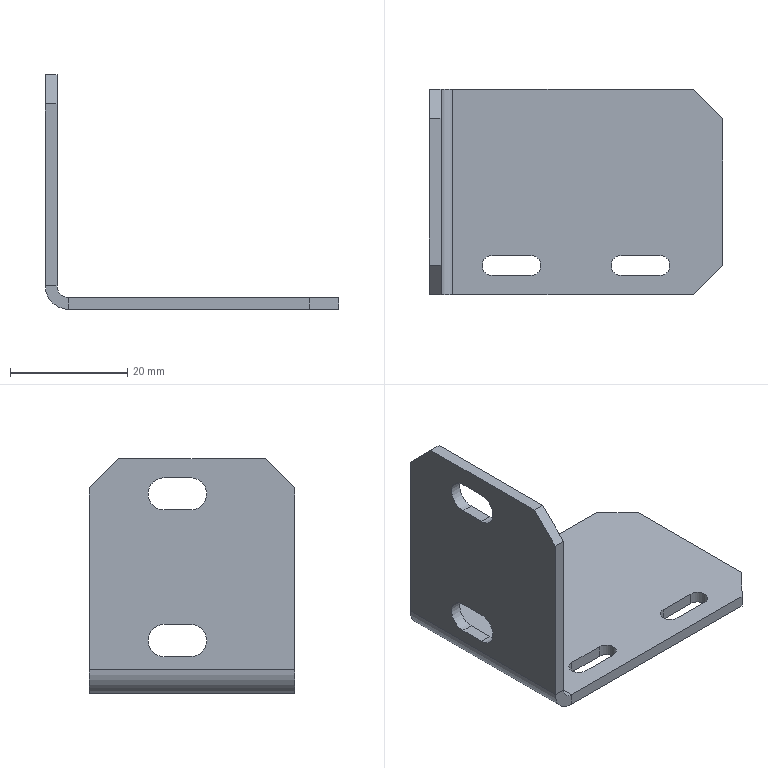Part | SolidWorks | features HoleWzd 2, Chamfer 1, EdgeFlange 1, FlatPattern 1, SMBaseFlange 1, SheetMetal 1 | 1 solid | 34 faces | box 50 x 35 x 40 mm | volume 5650 mm3 | plane 24 | cylinder 10 | commonest cylinder face diameters 3.4 x4 5.5 x4 4 x1 8 x1
STEP:
#1=CARTESIAN_POINT('',(48.,12.5,-20.));
#2=VERTEX_POINT('',#1);
#3=CARTESIAN_POINT('',(48.,-12.5,-20.));
#4=VERTEX_POINT('',#3);
#5=CARTESIAN_POINT('',(48.,0.,-20.));
#6=DIRECTION('',(0.,-1.,0.));
#7=VECTOR('',#6,1000.);
#8=LINE('',#5,#7);
#9=EDGE_CURVE('',#2,#4,#8,.T.);
#10=ORIENTED_EDGE('',*,*,#9,.T.);
#11=CARTESIAN_POINT('',(43.,-17.5,-20.));
#12=VERTEX_POINT('',#11);
#13=CARTESIAN_POINT('',(43.,-17.5,-20.));
#14=DIRECTION('',(-0.7071,-0.7071,0.));
#15=VECTOR('',#14,1000.);
#16=LINE('',#13,#15);
#17=EDGE_CURVE('',#4,#12,#16,.T.);
#18=ORIENTED_EDGE('',*,*,#17,.T.);
#19=CARTESIAN_POINT('',(2.,-17.5,-20.));
#20=VERTEX_POINT('',#19);
#21=CARTESIAN_POINT('',(0.,-17.5,-20.));
#22=DIRECTION('',(-1.,0.,0.));
#23=VECTOR('',#22,1000.);
#24=LINE('',#21,#23);
#25=EDGE_CURVE('',#12,#20,#24,.T.);
#26=ORIENTED_EDGE('',*,*,#25,.T.);
#27=CARTESIAN_POINT('',(2.,17.5,-20.));
#28=VERTEX_POINT('',#27);
#29=CARTESIAN_POINT('',(2.,-17.5,-20.));
#30=DIRECTION('',(0.,-1.,0.));
#31=VECTOR('',#30,1000.);
#32=LINE('',#29,#31);
#33=EDGE_CURVE('',#28,#20,#32,.T.);
#34=ORIENTED_EDGE('',*,*,#33,.F.);
#35=CARTESIAN_POINT('',(43.,17.5,-20.));
#36=VERTEX_POINT('',#35);
#37=CARTESIAN_POINT('',(0.,17.5,-20.));
#38=DIRECTION('',(1.,0.,0.));
#39=VECTOR('',#38,1000.);
#40=LINE('',#37,#39);
#41=EDGE_CURVE('',#28,#36,#40,.T.);
#42=ORIENTED_EDGE('',*,*,#41,.T.);
#43=CARTESIAN_POINT('',(48.,12.5,-20.));
#44=DIRECTION('',(0.7071,-0.7071,0.));
#45=VECTOR('',#44,1000.);
#46=LINE('',#43,#45);
#47=EDGE_CURVE('',#36,#2,#46,.T.);
#48=ORIENTED_EDGE('',*,*,#47,.T.);
#49=EDGE_LOOP('',(#10,#18,#26,#34,#42,#48));
#50=FACE_OUTER_BOUND('',#49,.T.);
#51=CARTESIAN_POINT('',(15.3,-10.8,-20.));
#52=VERTEX_POINT('',#51);
#53=CARTESIAN_POINT('',(8.7,-10.8,-20.));
#54=VERTEX_POINT('',#53);
#55=CARTESIAN_POINT('',(15.3,-10.8,-20.));
#56=DIRECTION('',(-1.,0.,0.));
#57=VECTOR('',#56,1000.);
#58=LINE('',#55,#57);
#59=EDGE_CURVE('',#52,#54,#58,.T.);
#60=ORIENTED_EDGE('',*,*,#59,.T.);
#61=CARTESIAN_POINT('',(8.7,-14.2,-20.));
#62=VERTEX_POINT('',#61);
#63=CARTESIAN_POINT('',(8.7,-12.5,-20.));
#64=DIRECTION('',(0.,0.,-1.));
#65=DIRECTION('',(0.,1.,0.));
#66=AXIS2_PLACEMENT_3D('',#63,#64,#65);
#67=CIRCLE('',#66,1.7);
#68=EDGE_CURVE('',#62,#54,#67,.T.);
#69=ORIENTED_EDGE('',*,*,#68,.F.);
#70=CARTESIAN_POINT('',(15.3,-14.2,-20.));
#71=VERTEX_POINT('',#70);
#72=CARTESIAN_POINT('',(15.3,-14.2,-20.));
#73=DIRECTION('',(-1.,0.,0.));
#74=VECTOR('',#73,1000.);
#75=LINE('',#72,#74);
#76=EDGE_CURVE('',#71,#62,#75,.T.);
#77=ORIENTED_EDGE('',*,*,#76,.F.);
#78=CARTESIAN_POINT('',(15.3,-12.5,-20.));
#79=DIRECTION('',(0.,0.,-1.));
#80=DIRECTION('',(0.,1.,0.));
#81=AXIS2_PLACEMENT_3D('',#78,#79,#80);
#82=CIRCLE('',#81,1.7);
#83=EDGE_CURVE('',#52,#71,#82,.T.);
#84=ORIENTED_EDGE('',*,*,#83,.F.);
#85=EDGE_LOOP('',(#60,#69,#77,#84));
#86=FACE_BOUND('',#85,.T.);
#87=CARTESIAN_POINT('',(37.3,-10.8,-20.));
#88=VERTEX_POINT('',#87);
#89=CARTESIAN_POINT('',(37.3,-14.2,-20.));
#90=VERTEX_POINT('',#89);
#91=CARTESIAN_POINT('',(37.3,-12.5,-20.));
#92=DIRECTION('',(0.,0.,-1.));
#93=DIRECTION('',(0.,1.,0.));
#94=AXIS2_PLACEMENT_3D('',#91,#92,#93);
#95=CIRCLE('',#94,1.7);
#96=EDGE_CURVE('',#88,#90,#95,.T.);
#97=ORIENTED_EDGE('',*,*,#96,.F.);
#98=CARTESIAN_POINT('',(30.7,-10.8,-20.));
#99=VERTEX_POINT('',#98);
#100=CARTESIAN_POINT('',(37.3,-10.8,-20.));
#101=DIRECTION('',(-1.,0.,0.));
#102=VECTOR('',#101,1000.);
#103=LINE('',#100,#102);
#104=EDGE_CURVE('',#88,#99,#103,.T.);
#105=ORIENTED_EDGE('',*,*,#104,.T.);
#106=CARTESIAN_POINT('',(30.7,-14.2,-20.));
#107=VERTEX_POINT('',#106);
#108=CARTESIAN_POINT('',(30.7,-12.5,-20.));
#109=DIRECTION('',(0.,0.,-1.));
#110=DIRECTION('',(0.,1.,0.));
#111=AXIS2_PLACEMENT_3D('',#108,#109,#110);
#112=CIRCLE('',#111,1.7);
#113=EDGE_CURVE('',#107,#99,#112,.T.);
#114=ORIENTED_EDGE('',*,*,#113,.F.);
#115=CARTESIAN_POINT('',(37.3,-14.2,-20.));
#116=DIRECTION('',(-1.,0.,0.));
#117=VECTOR('',#116,1000.);
#118=LINE('',#115,#117);
#119=EDGE_CURVE('',#90,#107,#118,.T.);
#120=ORIENTED_EDGE('',*,*,#119,.F.);
#121=EDGE_LOOP('',(#97,#105,#114,#120));
#122=FACE_BOUND('',#121,.T.);
#123=CARTESIAN_POINT('',(0.,0.,-20.));
#124=DIRECTION('',(0.,0.,1.));
#125=DIRECTION('',(1.,0.,0.));
#126=AXIS2_PLACEMENT_3D('',#123,#124,#125);
#127=PLANE('',#126);
#128=ADVANCED_FACE('',(#50,#86,#122),#127,.F.);
#129=CARTESIAN_POINT('',(-2.,17.5,-16.));
#130=VERTEX_POINT('',#129);
#131=CARTESIAN_POINT('',(-2.,17.5,15.));
#132=VERTEX_POINT('',#131);
#133=CARTESIAN_POINT('',(-2.,17.5,20.));
#134=DIRECTION('',(0.,0.,1.));
#135=VECTOR('',#134,1000.);
#136=LINE('',#133,#135);
#137=EDGE_CURVE('',#130,#132,#136,.T.);
#138=ORIENTED_EDGE('',*,*,#137,.T.);
#139=CARTESIAN_POINT('',(0.,17.5,15.));
#140=VERTEX_POINT('',#139);
#141=CARTESIAN_POINT('',(-2.,17.5,15.));
#142=DIRECTION('',(1.,0.,0.));
#143=VECTOR('',#142,1000.);
#144=LINE('',#141,#143);
#145=EDGE_CURVE('',#132,#140,#144,.T.);
#146=ORIENTED_EDGE('',*,*,#145,.T.);
#147=CARTESIAN_POINT('',(0.,17.5,-16.));
#148=VERTEX_POINT('',#147);
#149=CARTESIAN_POINT('',(0.,17.5,20.));
#150=DIRECTION('',(0.,0.,1.));
#151=VECTOR('',#150,1000.);
#152=LINE('',#149,#151);
#153=EDGE_CURVE('',#148,#140,#152,.T.);
#154=ORIENTED_EDGE('',*,*,#153,.F.);
#155=CARTESIAN_POINT('',(0.,17.5,-16.));
#156=DIRECTION('',(-1.,0.,0.));
#157=VECTOR('',#156,1000.);
#158=LINE('',#155,#157);
#159=EDGE_CURVE('',#148,#130,#158,.T.);
#160=ORIENTED_EDGE('',*,*,#159,.T.);
#161=EDGE_LOOP('',(#138,#146,#154,#160));
#162=FACE_OUTER_BOUND('',#161,.T.);
#163=CARTESIAN_POINT('',(-2.,17.5,20.));
#164=DIRECTION('',(0.,1.,0.));
#165=DIRECTION('',(0.,0.,1.));
#166=AXIS2_PLACEMENT_3D('',#163,#164,#165);
#167=PLANE('',#166);
#168=ADVANCED_FACE('',(#162),#167,.T.);
#169=CARTESIAN_POINT('',(-2.,4.75,16.75));
#170=VERTEX_POINT('',#169);
#171=CARTESIAN_POINT('',(-2.,0.25,16.75));
#172=VERTEX_POINT('',#171);
#173=CARTESIAN_POINT('',(-2.,4.75,16.75));
#174=DIRECTION('',(0.,-1.,0.));
#175=VECTOR('',#174,1000.);
#176=LINE('',#173,#175);
#177=EDGE_CURVE('',#170,#172,#176,.T.);
#178=ORIENTED_EDGE('',*,*,#177,.T.);
#179=CARTESIAN_POINT('',(-2.,0.25,11.25));
#180=VERTEX_POINT('',#179);
#181=CARTESIAN_POINT('',(-2.,0.25,14.));
#182=DIRECTION('',(1.,0.,0.));
#183=DIRECTION('',(0.,0.,-1.));
#184=AXIS2_PLACEMENT_3D('',#181,#182,#183);
#185=CIRCLE('',#184,2.75);
#186=EDGE_CURVE('',#172,#180,#185,.T.);
#187=ORIENTED_EDGE('',*,*,#186,.T.);
#188=CARTESIAN_POINT('',(-2.,4.75,11.25));
#189=VERTEX_POINT('',#188);
#190=CARTESIAN_POINT('',(-2.,4.75,11.25));
#191=DIRECTION('',(0.,-1.,0.));
#192=VECTOR('',#191,1000.);
#193=LINE('',#190,#192);
#194=EDGE_CURVE('',#189,#180,#193,.T.);
#195=ORIENTED_EDGE('',*,*,#194,.F.);
#196=CARTESIAN_POINT('',(-2.,4.75,14.));
#197=DIRECTION('',(1.,0.,0.));
#198=DIRECTION('',(0.,0.,-1.));
#199=AXIS2_PLACEMENT_3D('',#196,#197,#198);
#200=CIRCLE('',#199,2.75);
#201=EDGE_CURVE('',#189,#170,#200,.T.);
#202=ORIENTED_EDGE('',*,*,#201,.T.);
#203=EDGE_LOOP('',(#178,#187,#195,#202));
#204=FACE_BOUND('',#203,.T.);
#205=CARTESIAN_POINT('',(-2.,4.75,-8.25));
#206=VERTEX_POINT('',#205);
#207=CARTESIAN_POINT('',(-2.,0.25,-8.25));
#208=VERTEX_POINT('',#207);
#209=CARTESIAN_POINT('',(-2.,4.75,-8.25));
#210=DIRECTION('',(0.,-1.,0.));
#211=VECTOR('',#210,1000.);
#212=LINE('',#209,#211);
#213=EDGE_CURVE('',#206,#208,#212,.T.);
#214=ORIENTED_EDGE('',*,*,#213,.T.);
#215=CARTESIAN_POINT('',(-2.,0.25,-13.75));
#216=VERTEX_POINT('',#215);
#217=CARTESIAN_POINT('',(-2.,0.25,-11.));
#218=DIRECTION('',(1.,0.,0.));
#219=DIRECTION('',(0.,0.,-1.));
#220=AXIS2_PLACEMENT_3D('',#217,#218,#219);
#221=CIRCLE('',#220,2.75);
#222=EDGE_CURVE('',#208,#216,#221,.T.);
#223=ORIENTED_EDGE('',*,*,#222,.T.);
#224=CARTESIAN_POINT('',(-2.,4.75,-13.75));
#225=VERTEX_POINT('',#224);
#226=CARTESIAN_POINT('',(-2.,4.75,-13.75));
#227=DIRECTION('',(0.,-1.,0.));
#228=VECTOR('',#227,1000.);
#229=LINE('',#226,#228);
#230=EDGE_CURVE('',#225,#216,#229,.T.);
#231=ORIENTED_EDGE('',*,*,#230,.F.);
#232=CARTESIAN_POINT('',(-2.,4.75,-11.));
#233=DIRECTION('',(1.,0.,0.));
#234=DIRECTION('',(0.,0.,-1.));
#235=AXIS2_PLACEMENT_3D('',#232,#233,#234);
#236=CIRCLE('',#235,2.75);
#237=EDGE_CURVE('',#225,#206,#236,.T.);
#238=ORIENTED_EDGE('',*,*,#237,.T.);
#239=EDGE_LOOP('',(#214,#223,#231,#238));
#240=FACE_BOUND('',#239,.T.);
#241=CARTESIAN_POINT('',(-2.,-17.5,15.));
#242=VERTEX_POINT('',#241);
#243=CARTESIAN_POINT('',(-2.,-17.5,-16.));
#244=VERTEX_POINT('',#243);
#245=CARTESIAN_POINT('',(-2.,-17.5,20.));
#246=DIRECTION('',(0.,0.,-1.));
#247=VECTOR('',#246,1000.);
#248=LINE('',#245,#247);
#249=EDGE_CURVE('',#242,#244,#248,.T.);
#250=ORIENTED_EDGE('',*,*,#249,.F.);
#251=CARTESIAN_POINT('',(-2.,-12.5,20.));
#252=VERTEX_POINT('',#251);
#253=CARTESIAN_POINT('',(-2.,-12.5,20.));
#254=DIRECTION('',(0.,0.7071,0.7071));
#255=VECTOR('',#254,1000.);
#256=LINE('',#253,#255);
#257=EDGE_CURVE('',#242,#252,#256,.T.);
#258=ORIENTED_EDGE('',*,*,#257,.T.);
#259=CARTESIAN_POINT('',(-2.,12.5,20.));
#260=VERTEX_POINT('',#259);
#261=CARTESIAN_POINT('',(-2.,17.5,20.));
#262=DIRECTION('',(0.,-1.,0.));
#263=VECTOR('',#262,1000.);
#264=LINE('',#261,#263);
#265=EDGE_CURVE('',#260,#252,#264,.T.);
#266=ORIENTED_EDGE('',*,*,#265,.F.);
#267=CARTESIAN_POINT('',(-2.,17.5,15.));
#268=DIRECTION('',(0.,0.7071,-0.7071));
#269=VECTOR('',#268,1000.);
#270=LINE('',#267,#269);
#271=EDGE_CURVE('',#260,#132,#270,.T.);
#272=ORIENTED_EDGE('',*,*,#271,.T.);
#273=ORIENTED_EDGE('',*,*,#137,.F.);
#274=CARTESIAN_POINT('',(-2.,17.5,-16.));
#275=DIRECTION('',(0.,-1.,0.));
#276=VECTOR('',#275,1000.);
#277=LINE('',#274,#276);
#278=EDGE_CURVE('',#130,#244,#277,.T.);
#279=ORIENTED_EDGE('',*,*,#278,.T.);
#280=EDGE_LOOP('',(#250,#258,#266,#272,#273,#279));
#281=FACE_OUTER_BOUND('',#280,.T.);
#282=CARTESIAN_POINT('',(-2.,0.,0.));
#283=DIRECTION('',(1.,0.,0.));
#284=DIRECTION('',(0.,0.,-1.));
#285=AXIS2_PLACEMENT_3D('',#282,#283,#284);
#286=PLANE('',#285);
#287=ADVANCED_FACE('',(#204,#240,#281),#286,.F.);
#288=CARTESIAN_POINT('',(0.,4.75,11.25));
#289=VERTEX_POINT('',#288);
#290=CARTESIAN_POINT('',(0.,0.25,11.25));
#291=VERTEX_POINT('',#290);
#292=CARTESIAN_POINT('',(0.,4.75,11.25));
#293=DIRECTION('',(0.,-1.,0.));
#294=VECTOR('',#293,1000.);
#295=LINE('',#292,#294);
#296=EDGE_CURVE('',#289,#291,#295,.T.);
#297=ORIENTED_EDGE('',*,*,#296,.T.);
#298=CARTESIAN_POINT('',(0.,0.25,16.75));
#299=VERTEX_POINT('',#298);
#300=CARTESIAN_POINT('',(0.,0.25,14.));
#301=DIRECTION('',(1.,0.,0.));
#302=DIRECTION('',(0.,0.,-1.));
#303=AXIS2_PLACEMENT_3D('',#300,#301,#302);
#304=CIRCLE('',#303,2.75);
#305=EDGE_CURVE('',#299,#291,#304,.T.);
#306=ORIENTED_EDGE('',*,*,#305,.F.);
#307=CARTESIAN_POINT('',(0.,4.75,16.75));
#308=VERTEX_POINT('',#307);
#309=CARTESIAN_POINT('',(0.,4.75,16.75));
#310=DIRECTION('',(0.,-1.,0.));
#311=VECTOR('',#310,1000.);
#312=LINE('',#309,#311);
#313=EDGE_CURVE('',#308,#299,#312,.T.);
#314=ORIENTED_EDGE('',*,*,#313,.F.);
#315=CARTESIAN_POINT('',(0.,4.75,14.));
#316=DIRECTION('',(1.,0.,0.));
#317=DIRECTION('',(0.,0.,-1.));
#318=AXIS2_PLACEMENT_3D('',#315,#316,#317);
#319=CIRCLE('',#318,2.75);
#320=EDGE_CURVE('',#289,#308,#319,.T.);
#321=ORIENTED_EDGE('',*,*,#320,.F.);
#322=EDGE_LOOP('',(#297,#306,#314,#321));
#323=FACE_BOUND('',#322,.T.);
#324=CARTESIAN_POINT('',(0.,4.75,-13.75));
#325=VERTEX_POINT('',#324);
#326=CARTESIAN_POINT('',(0.,0.25,-13.75));
#327=VERTEX_POINT('',#326);
#328=CARTESIAN_POINT('',(0.,4.75,-13.75));
#329=DIRECTION('',(0.,-1.,0.));
#330=VECTOR('',#329,1000.);
#331=LINE('',#328,#330);
#332=EDGE_CURVE('',#325,#327,#331,.T.);
#333=ORIENTED_EDGE('',*,*,#332,.T.);
#334=CARTESIAN_POINT('',(0.,0.25,-8.25));
#335=VERTEX_POINT('',#334);
#336=CARTESIAN_POINT('',(0.,0.25,-11.));
#337=DIRECTION('',(1.,0.,0.));
#338=DIRECTION('',(0.,0.,-1.));
#339=AXIS2_PLACEMENT_3D('',#336,#337,#338);
#340=CIRCLE('',#339,2.75);
#341=EDGE_CURVE('',#335,#327,#340,.T.);
#342=ORIENTED_EDGE('',*,*,#341,.F.);
#343=CARTESIAN_POINT('',(0.,4.75,-8.25));
#344=VERTEX_POINT('',#343);
#345=CARTESIAN_POINT('',(0.,4.75,-8.25));
#346=DIRECTION('',(0.,-1.,0.));
#347=VECTOR('',#346,1000.);
#348=LINE('',#345,#347);
#349=EDGE_CURVE('',#344,#335,#348,.T.);
#350=ORIENTED_EDGE('',*,*,#349,.F.);
#351=CARTESIAN_POINT('',(0.,4.75,-11.));
#352=DIRECTION('',(1.,0.,0.));
#353=DIRECTION('',(0.,0.,-1.));
#354=AXIS2_PLACEMENT_3D('',#351,#352,#353);
#355=CIRCLE('',#354,2.75);
#356=EDGE_CURVE('',#325,#344,#355,.T.);
#357=ORIENTED_EDGE('',*,*,#356,.F.);
#358=EDGE_LOOP('',(#333,#342,#350,#357));
#359=FACE_BOUND('',#358,.T.);
#360=CARTESIAN_POINT('',(0.,12.5,20.));
#361=VERTEX_POINT('',#360);
#362=CARTESIAN_POINT('',(0.,-12.5,20.));
#363=VERTEX_POINT('',#362);
#364=CARTESIAN_POINT('',(0.,17.5,20.));
#365=DIRECTION('',(0.,-1.,0.));
#366=VECTOR('',#365,1000.);
#367=LINE('',#364,#366);
#368=EDGE_CURVE('',#361,#363,#367,.T.);
#369=ORIENTED_EDGE('',*,*,#368,.T.);
#370=CARTESIAN_POINT('',(0.,-17.5,15.));
#371=VERTEX_POINT('',#370);
#372=CARTESIAN_POINT('',(0.,-16.25,16.25));
#373=DIRECTION('',(0.,-0.7071,-0.7071));
#374=VECTOR('',#373,1000.);
#375=LINE('',#372,#374);
#376=EDGE_CURVE('',#363,#371,#375,.T.);
#377=ORIENTED_EDGE('',*,*,#376,.T.);
#378=CARTESIAN_POINT('',(0.,-17.5,-16.));
#379=VERTEX_POINT('',#378);
#380=CARTESIAN_POINT('',(0.,-17.5,20.));
#381=DIRECTION('',(0.,0.,-1.));
#382=VECTOR('',#381,1000.);
#383=LINE('',#380,#382);
#384=EDGE_CURVE('',#371,#379,#383,.T.);
#385=ORIENTED_EDGE('',*,*,#384,.T.);
#386=CARTESIAN_POINT('',(0.,17.5,-16.));
#387=DIRECTION('',(0.,-1.,0.));
#388=VECTOR('',#387,1000.);
#389=LINE('',#386,#388);
#390=EDGE_CURVE('',#148,#379,#389,.T.);
#391=ORIENTED_EDGE('',*,*,#390,.F.);
#392=ORIENTED_EDGE('',*,*,#153,.T.);
#393=CARTESIAN_POINT('',(0.,16.25,16.25));
#394=DIRECTION('',(0.,-0.7071,0.7071));
#395=VECTOR('',#394,1000.);
#396=LINE('',#393,#395);
#397=EDGE_CURVE('',#140,#361,#396,.T.);
#398=ORIENTED_EDGE('',*,*,#397,.T.);
#399=EDGE_LOOP('',(#369,#377,#385,#391,#392,#398));
#400=FACE_OUTER_BOUND('',#399,.T.);
#401=CARTESIAN_POINT('',(0.,0.,0.));
#402=DIRECTION('',(1.,0.,0.));
#403=DIRECTION('',(0.,0.,-1.));
#404=AXIS2_PLACEMENT_3D('',#401,#402,#403);
#405=PLANE('',#404);
#406=ADVANCED_FACE('',(#323,#359,#400),#405,.T.);
#407=ORIENTED_EDGE('',*,*,#384,.F.);
#408=CARTESIAN_POINT('',(-2.,-17.5,15.));
#409=DIRECTION('',(-1.,0.,0.));
#410=VECTOR('',#409,1000.);
#411=LINE('',#408,#410);
#412=EDGE_CURVE('',#371,#242,#411,.T.);
#413=ORIENTED_EDGE('',*,*,#412,.T.);
#414=ORIENTED_EDGE('',*,*,#249,.T.);
#415=CARTESIAN_POINT('',(0.,-17.5,-16.));
#416=DIRECTION('',(-1.,0.,0.));
#417=VECTOR('',#416,1000.);
#418=LINE('',#415,#417);
#419=EDGE_CURVE('',#379,#244,#418,.T.);
#420=ORIENTED_EDGE('',*,*,#419,.F.);
#421=EDGE_LOOP('',(#407,#413,#414,#420));
#422=FACE_OUTER_BOUND('',#421,.T.);
#423=CARTESIAN_POINT('',(-2.,-17.5,20.));
#424=DIRECTION('',(0.,-1.,0.));
#425=DIRECTION('',(0.,0.,-1.));
#426=AXIS2_PLACEMENT_3D('',#423,#424,#425);
#427=PLANE('',#426);
#428=ADVANCED_FACE('',(#422),#427,.T.);
#429=ORIENTED_EDGE('',*,*,#265,.T.);
#430=CARTESIAN_POINT('',(-2.,-12.5,20.));
#431=DIRECTION('',(1.,0.,0.));
#432=VECTOR('',#431,1000.);
#433=LINE('',#430,#432);
#434=EDGE_CURVE('',#252,#363,#433,.T.);
#435=ORIENTED_EDGE('',*,*,#434,.T.);
#436=ORIENTED_EDGE('',*,*,#368,.F.);
#437=CARTESIAN_POINT('',(-2.,12.5,20.));
#438=DIRECTION('',(-1.,0.,0.));
#439=VECTOR('',#438,1000.);
#440=LINE('',#437,#439);
#441=EDGE_CURVE('',#361,#260,#440,.T.);
#442=ORIENTED_EDGE('',*,*,#441,.T.);
#443=EDGE_LOOP('',(#429,#435,#436,#442));
#444=FACE_OUTER_BOUND('',#443,.T.);
#445=CARTESIAN_POINT('',(-2.,17.5,20.));
#446=DIRECTION('',(0.,0.,1.));
#447=DIRECTION('',(0.,-1.,0.));
#448=AXIS2_PLACEMENT_3D('',#445,#446,#447);
#449=PLANE('',#448);
#450=ADVANCED_FACE('',(#444),#449,.T.);
#451=CARTESIAN_POINT('',(2.,-17.5,-18.));
#452=VERTEX_POINT('',#451);
#453=CARTESIAN_POINT('',(2.,-17.5,-20.));
#454=DIRECTION('',(0.,0.,-1.));
#455=VECTOR('',#454,1000.);
#456=LINE('',#453,#455);
#457=EDGE_CURVE('',#452,#20,#456,.T.);
#458=ORIENTED_EDGE('',*,*,#457,.F.);
#459=CARTESIAN_POINT('',(2.,-17.5,-16.));
#460=DIRECTION('',(0.,-1.,0.));
#461=DIRECTION('',(0.,0.,1.));
#462=AXIS2_PLACEMENT_3D('',#459,#460,#461);
#463=CIRCLE('',#462,2.);
#464=EDGE_CURVE('',#379,#452,#463,.T.);
#465=ORIENTED_EDGE('',*,*,#464,.F.);
#466=ORIENTED_EDGE('',*,*,#419,.T.);
#467=CARTESIAN_POINT('',(2.,-17.5,-16.));
#468=DIRECTION('',(0.,-1.,0.));
#469=DIRECTION('',(0.,0.,1.));
#470=AXIS2_PLACEMENT_3D('',#467,#468,#469);
#471=CIRCLE('',#470,4.);
#472=EDGE_CURVE('',#244,#20,#471,.T.);
#473=ORIENTED_EDGE('',*,*,#472,.T.);
#474=EDGE_LOOP('',(#458,#465,#466,#473));
#475=FACE_OUTER_BOUND('',#474,.T.);
#476=CARTESIAN_POINT('',(2.,-17.5,-16.));
#477=DIRECTION('',(0.,-1.,0.));
#478=DIRECTION('',(0.,0.,-1.));
#479=AXIS2_PLACEMENT_3D('',#476,#477,#478);
#480=PLANE('',#479);
#481=ADVANCED_FACE('',(#475),#480,.T.);
#482=CARTESIAN_POINT('',(2.,17.5,-18.));
#483=VERTEX_POINT('',#482);
#484=CARTESIAN_POINT('',(2.,17.5,-16.));
#485=DIRECTION('',(0.,1.,0.));
#486=DIRECTION('',(0.,0.,1.));
#487=AXIS2_PLACEMENT_3D('',#484,#485,#486);
#488=CIRCLE('',#487,2.);
#489=EDGE_CURVE('',#483,#148,#488,.T.);
#490=ORIENTED_EDGE('',*,*,#489,.F.);
#491=CARTESIAN_POINT('',(2.,17.5,-18.));
#492=DIRECTION('',(0.,0.,-1.));
#493=VECTOR('',#492,1000.);
#494=LINE('',#491,#493);
#495=EDGE_CURVE('',#483,#28,#494,.T.);
#496=ORIENTED_EDGE('',*,*,#495,.T.);
#497=CARTESIAN_POINT('',(2.,17.5,-16.));
#498=DIRECTION('',(0.,1.,0.));
#499=DIRECTION('',(0.,0.,1.));
#500=AXIS2_PLACEMENT_3D('',#497,#498,#499);
#501=CIRCLE('',#500,4.);
#502=EDGE_CURVE('',#28,#130,#501,.T.);
#503=ORIENTED_EDGE('',*,*,#502,.T.);
#504=ORIENTED_EDGE('',*,*,#159,.F.);
#505=EDGE_LOOP('',(#490,#496,#503,#504));
#506=FACE_OUTER_BOUND('',#505,.T.);
#507=CARTESIAN_POINT('',(2.,17.5,-16.));
#508=DIRECTION('',(0.,-1.,0.));
#509=DIRECTION('',(0.,0.,-1.));
#510=AXIS2_PLACEMENT_3D('',#507,#508,#509);
#511=PLANE('',#510);
#512=ADVANCED_FACE('',(#506),#511,.F.);
#513=ORIENTED_EDGE('',*,*,#278,.F.);
#514=ORIENTED_EDGE('',*,*,#502,.F.);
#515=ORIENTED_EDGE('',*,*,#33,.T.);
#516=ORIENTED_EDGE('',*,*,#472,.F.);
#517=EDGE_LOOP('',(#513,#514,#515,#516));
#518=FACE_OUTER_BOUND('',#517,.T.);
#519=CARTESIAN_POINT('',(2.,17.5,-16.));
#520=DIRECTION('',(0.,1.,0.));
#521=DIRECTION('',(0.,0.,-1.));
#522=AXIS2_PLACEMENT_3D('',#519,#520,#521);
#523=CYLINDRICAL_SURFACE('',#522,4.);
#524=ADVANCED_FACE('',(#518),#523,.T.);
#525=ORIENTED_EDGE('',*,*,#390,.T.);
#526=ORIENTED_EDGE('',*,*,#464,.T.);
#527=CARTESIAN_POINT('',(2.,-17.5,-18.));
#528=DIRECTION('',(0.,1.,0.));
#529=VECTOR('',#528,1000.);
#530=LINE('',#527,#529);
#531=EDGE_CURVE('',#452,#483,#530,.T.);
#532=ORIENTED_EDGE('',*,*,#531,.T.);
#533=ORIENTED_EDGE('',*,*,#489,.T.);
#534=EDGE_LOOP('',(#525,#526,#532,#533));
#535=FACE_OUTER_BOUND('',#534,.T.);
#536=CARTESIAN_POINT('',(2.,17.5,-16.));
#537=DIRECTION('',(0.,1.,0.));
#538=DIRECTION('',(0.,0.,-1.));
#539=AXIS2_PLACEMENT_3D('',#536,#537,#538);
#540=CYLINDRICAL_SURFACE('',#539,2.);
#541=ADVANCED_FACE('',(#535),#540,.F.);
#542=ORIENTED_EDGE('',*,*,#25,.F.);
#543=CARTESIAN_POINT('',(43.,-17.5,-18.));
#544=VERTEX_POINT('',#543);
#545=CARTESIAN_POINT('',(43.,-17.5,-20.));
#546=DIRECTION('',(0.,0.,1.));
#547=VECTOR('',#546,1000.);
#548=LINE('',#545,#547);
#549=EDGE_CURVE('',#12,#544,#548,.T.);
#550=ORIENTED_EDGE('',*,*,#549,.T.);
#551=CARTESIAN_POINT('',(0.,-17.5,-18.));
#552=DIRECTION('',(-1.,0.,0.));
#553=VECTOR('',#552,1000.);
#554=LINE('',#551,#553);
#555=EDGE_CURVE('',#544,#452,#554,.T.);
#556=ORIENTED_EDGE('',*,*,#555,.T.);
#557=ORIENTED_EDGE('',*,*,#457,.T.);
#558=EDGE_LOOP('',(#542,#550,#556,#557));
#559=FACE_OUTER_BOUND('',#558,.T.);
#560=CARTESIAN_POINT('',(0.,-17.5,-20.));
#561=DIRECTION('',(0.,1.,0.));
#562=DIRECTION('',(0.,0.,1.));
#563=AXIS2_PLACEMENT_3D('',#560,#561,#562);
#564=PLANE('',#563);
#565=ADVANCED_FACE('',(#559),#564,.F.);
#566=CARTESIAN_POINT('',(43.,17.5,-18.));
#567=VERTEX_POINT('',#566);
#568=CARTESIAN_POINT('',(48.,17.5,-18.));
#569=DIRECTION('',(1.,0.,0.));
#570=VECTOR('',#569,1000.);
#571=LINE('',#568,#570);
#572=EDGE_CURVE('',#483,#567,#571,.T.);
#573=ORIENTED_EDGE('',*,*,#572,.T.);
#574=CARTESIAN_POINT('',(43.,17.5,-20.));
#575=DIRECTION('',(0.,0.,-1.));
#576=VECTOR('',#575,1000.);
#577=LINE('',#574,#576);
#578=EDGE_CURVE('',#567,#36,#577,.T.);
#579=ORIENTED_EDGE('',*,*,#578,.T.);
#580=ORIENTED_EDGE('',*,*,#41,.F.);
#581=ORIENTED_EDGE('',*,*,#495,.F.);
#582=EDGE_LOOP('',(#573,#579,#580,#581));
#583=FACE_OUTER_BOUND('',#582,.T.);
#584=CARTESIAN_POINT('',(48.,17.5,-20.));
#585=DIRECTION('',(0.,-1.,0.));
#586=DIRECTION('',(1.,0.,0.));
#587=AXIS2_PLACEMENT_3D('',#584,#585,#586);
#588=PLANE('',#587);
#589=ADVANCED_FACE('',(#583),#588,.F.);
#590=CARTESIAN_POINT('',(37.3,-14.2,-18.));
#591=VERTEX_POINT('',#590);
#592=CARTESIAN_POINT('',(37.3,-10.8,-18.));
#593=VERTEX_POINT('',#592);
#594=CARTESIAN_POINT('',(37.3,-12.5,-18.));
#595=DIRECTION('',(0.,0.,1.));
#596=DIRECTION('',(1.,0.,0.));
#597=AXIS2_PLACEMENT_3D('',#594,#595,#596);
#598=CIRCLE('',#597,1.7);
#599=EDGE_CURVE('',#591,#593,#598,.T.);
#600=ORIENTED_EDGE('',*,*,#599,.F.);
#601=CARTESIAN_POINT('',(30.7,-14.2,-18.));
#602=VERTEX_POINT('',#601);
#603=CARTESIAN_POINT('',(0.,-14.2,-18.));
#604=DIRECTION('',(1.,0.,0.));
#605=VECTOR('',#604,1000.);
#606=LINE('',#603,#605);
#607=EDGE_CURVE('',#602,#591,#606,.T.);
#608=ORIENTED_EDGE('',*,*,#607,.F.);
#609=CARTESIAN_POINT('',(30.7,-10.8,-18.));
#610=VERTEX_POINT('',#609);
#611=CARTESIAN_POINT('',(30.7,-12.5,-18.));
#612=DIRECTION('',(0.,0.,1.));
#613=DIRECTION('',(1.,0.,0.));
#614=AXIS2_PLACEMENT_3D('',#611,#612,#613);
#615=CIRCLE('',#614,1.7);
#616=EDGE_CURVE('',#610,#602,#615,.T.);
#617=ORIENTED_EDGE('',*,*,#616,.F.);
#618=CARTESIAN_POINT('',(0.,-10.8,-18.));
#619=DIRECTION('',(-1.,0.,0.));
#620=VECTOR('',#619,1000.);
#621=LINE('',#618,#620);
#622=EDGE_CURVE('',#593,#610,#621,.T.);
#623=ORIENTED_EDGE('',*,*,#622,.F.);
#624=EDGE_LOOP('',(#600,#608,#617,#623));
#625=FACE_BOUND('',#624,.T.);
#626=CARTESIAN_POINT('',(8.7,-14.2,-18.));
#627=VERTEX_POINT('',#626);
#628=CARTESIAN_POINT('',(15.3,-14.2,-18.));
#629=VERTEX_POINT('',#628);
#630=CARTESIAN_POINT('',(0.,-14.2,-18.));
#631=DIRECTION('',(1.,0.,0.));
#632=VECTOR('',#631,1000.);
#633=LINE('',#630,#632);
#634=EDGE_CURVE('',#627,#629,#633,.T.);
#635=ORIENTED_EDGE('',*,*,#634,.F.);
#636=CARTESIAN_POINT('',(8.7,-10.8,-18.));
#637=VERTEX_POINT('',#636);
#638=CARTESIAN_POINT('',(8.7,-12.5,-18.));
#639=DIRECTION('',(0.,0.,1.));
#640=DIRECTION('',(1.,0.,0.));
#641=AXIS2_PLACEMENT_3D('',#638,#639,#640);
#642=CIRCLE('',#641,1.7);
#643=EDGE_CURVE('',#637,#627,#642,.T.);
#644=ORIENTED_EDGE('',*,*,#643,.F.);
#645=CARTESIAN_POINT('',(15.3,-10.8,-18.));
#646=VERTEX_POINT('',#645);
#647=CARTESIAN_POINT('',(0.,-10.8,-18.));
#648=DIRECTION('',(-1.,0.,0.));
#649=VECTOR('',#648,1000.);
#650=LINE('',#647,#649);
#651=EDGE_CURVE('',#646,#637,#650,.T.);
#652=ORIENTED_EDGE('',*,*,#651,.F.);
#653=CARTESIAN_POINT('',(15.3,-12.5,-18.));
#654=DIRECTION('',(0.,0.,1.));
#655=DIRECTION('',(1.,0.,0.));
#656=AXIS2_PLACEMENT_3D('',#653,#654,#655);
#657=CIRCLE('',#656,1.7);
#658=EDGE_CURVE('',#629,#646,#657,.T.);
#659=ORIENTED_EDGE('',*,*,#658,.F.);
#660=EDGE_LOOP('',(#635,#644,#652,#659));
#661=FACE_BOUND('',#660,.T.);
#662=ORIENTED_EDGE('',*,*,#555,.F.);
#663=CARTESIAN_POINT('',(48.,-12.5,-18.));
#664=VERTEX_POINT('',#663);
#665=CARTESIAN_POINT('',(30.25,-30.25,-18.));
#666=DIRECTION('',(0.7071,0.7071,0.));
#667=VECTOR('',#666,1000.);
#668=LINE('',#665,#667);
#669=EDGE_CURVE('',#544,#664,#668,.T.);
#670=ORIENTED_EDGE('',*,*,#669,.T.);
#671=CARTESIAN_POINT('',(48.,12.5,-18.));
#672=VERTEX_POINT('',#671);
#673=CARTESIAN_POINT('',(48.,-17.5,-18.));
#674=DIRECTION('',(0.,-1.,0.));
#675=VECTOR('',#674,1000.);
#676=LINE('',#673,#675);
#677=EDGE_CURVE('',#672,#664,#676,.T.);
#678=ORIENTED_EDGE('',*,*,#677,.F.);
#679=CARTESIAN_POINT('',(30.25,30.25,-18.));
#680=DIRECTION('',(-0.7071,0.7071,0.));
#681=VECTOR('',#680,1000.);
#682=LINE('',#679,#681);
#683=EDGE_CURVE('',#672,#567,#682,.T.);
#684=ORIENTED_EDGE('',*,*,#683,.T.);
#685=ORIENTED_EDGE('',*,*,#572,.F.);
#686=ORIENTED_EDGE('',*,*,#531,.F.);
#687=EDGE_LOOP('',(#662,#670,#678,#684,#685,#686));
#688=FACE_OUTER_BOUND('',#687,.T.);
#689=CARTESIAN_POINT('',(0.,0.,-18.));
#690=DIRECTION('',(0.,0.,1.));
#691=DIRECTION('',(1.,0.,0.));
#692=AXIS2_PLACEMENT_3D('',#689,#690,#691);
#693=PLANE('',#692);
#694=ADVANCED_FACE('',(#625,#661,#688),#693,.T.);
#695=ORIENTED_EDGE('',*,*,#677,.T.);
#696=CARTESIAN_POINT('',(48.,-12.5,-20.));
#697=DIRECTION('',(0.,0.,-1.));
#698=VECTOR('',#697,1000.);
#699=LINE('',#696,#698);
#700=EDGE_CURVE('',#664,#4,#699,.T.);
#701=ORIENTED_EDGE('',*,*,#700,.T.);
#702=ORIENTED_EDGE('',*,*,#9,.F.);
#703=CARTESIAN_POINT('',(48.,12.5,-20.));
#704=DIRECTION('',(0.,0.,1.));
#705=VECTOR('',#704,1000.);
#706=LINE('',#703,#705);
#707=EDGE_CURVE('',#2,#672,#706,.T.);
#708=ORIENTED_EDGE('',*,*,#707,.T.);
#709=EDGE_LOOP('',(#695,#701,#702,#708));
#710=FACE_OUTER_BOUND('',#709,.T.);
#711=CARTESIAN_POINT('',(48.,-17.5,-20.));
#712=DIRECTION('',(-1.,0.,0.));
#713=DIRECTION('',(0.,0.,1.));
#714=AXIS2_PLACEMENT_3D('',#711,#712,#713);
#715=PLANE('',#714);
#716=ADVANCED_FACE('',(#710),#715,.F.);
#717=ORIENTED_EDGE('',*,*,#257,.F.);
#718=ORIENTED_EDGE('',*,*,#412,.F.);
#719=ORIENTED_EDGE('',*,*,#376,.F.);
#720=ORIENTED_EDGE('',*,*,#434,.F.);
#721=EDGE_LOOP('',(#717,#718,#719,#720));
#722=FACE_OUTER_BOUND('',#721,.T.);
#723=CARTESIAN_POINT('',(-2.,-12.5,20.));
#724=DIRECTION('',(0.,0.7071,-0.7071));
#725=DIRECTION('',(1.,0.,0.));
#726=AXIS2_PLACEMENT_3D('',#723,#724,#725);
#727=PLANE('',#726);
#728=ADVANCED_FACE('',(#722),#727,.F.);
#729=ORIENTED_EDGE('',*,*,#271,.F.);
#730=ORIENTED_EDGE('',*,*,#441,.F.);
#731=ORIENTED_EDGE('',*,*,#397,.F.);
#732=ORIENTED_EDGE('',*,*,#145,.F.);
#733=EDGE_LOOP('',(#729,#730,#731,#732));
#734=FACE_OUTER_BOUND('',#733,.T.);
#735=CARTESIAN_POINT('',(-2.,17.5,15.));
#736=DIRECTION('',(0.,-0.7071,-0.7071));
#737=DIRECTION('',(1.,0.,0.));
#738=AXIS2_PLACEMENT_3D('',#735,#736,#737);
#739=PLANE('',#738);
#740=ADVANCED_FACE('',(#734),#739,.F.);
#741=ORIENTED_EDGE('',*,*,#17,.F.);
#742=ORIENTED_EDGE('',*,*,#700,.F.);
#743=ORIENTED_EDGE('',*,*,#669,.F.);
#744=ORIENTED_EDGE('',*,*,#549,.F.);
#745=EDGE_LOOP('',(#741,#742,#743,#744));
#746=FACE_OUTER_BOUND('',#745,.T.);
#747=CARTESIAN_POINT('',(43.,-17.5,-20.));
#748=DIRECTION('',(-0.7071,0.7071,0.));
#749=DIRECTION('',(0.,0.,1.));
#750=AXIS2_PLACEMENT_3D('',#747,#748,#749);
#751=PLANE('',#750);
#752=ADVANCED_FACE('',(#746),#751,.F.);
#753=ORIENTED_EDGE('',*,*,#47,.F.);
#754=ORIENTED_EDGE('',*,*,#578,.F.);
#755=ORIENTED_EDGE('',*,*,#683,.F.);
#756=ORIENTED_EDGE('',*,*,#707,.F.);
#757=EDGE_LOOP('',(#753,#754,#755,#756));
#758=FACE_OUTER_BOUND('',#757,.T.);
#759=CARTESIAN_POINT('',(48.,12.5,-20.));
#760=DIRECTION('',(-0.7071,-0.7071,0.));
#761=DIRECTION('',(0.,0.,1.));
#762=AXIS2_PLACEMENT_3D('',#759,#760,#761);
#763=PLANE('',#762);
#764=ADVANCED_FACE('',(#758),#763,.F.);
#765=ORIENTED_EDGE('',*,*,#341,.T.);
#766=CARTESIAN_POINT('',(0.,0.25,-13.75));
#767=DIRECTION('',(1.,0.,0.));
#768=VECTOR('',#767,1000.);
#769=LINE('',#766,#768);
#770=EDGE_CURVE('',#216,#327,#769,.T.);
#771=ORIENTED_EDGE('',*,*,#770,.F.);
#772=ORIENTED_EDGE('',*,*,#222,.F.);
#773=CARTESIAN_POINT('',(0.,0.25,-8.25));
#774=DIRECTION('',(-1.,0.,0.));
#775=VECTOR('',#774,1000.);
#776=LINE('',#773,#775);
#777=EDGE_CURVE('',#335,#208,#776,.T.);
#778=ORIENTED_EDGE('',*,*,#777,.F.);
#779=EDGE_LOOP('',(#765,#771,#772,#778));
#780=FACE_OUTER_BOUND('',#779,.T.);
#781=CARTESIAN_POINT('',(0.,0.25,-11.));
#782=DIRECTION('',(1.,0.,0.));
#783=DIRECTION('',(0.,0.,-1.));
#784=AXIS2_PLACEMENT_3D('',#781,#782,#783);
#785=CYLINDRICAL_SURFACE('',#784,2.75);
#786=ADVANCED_FACE('',(#780),#785,.F.);
#787=ORIENTED_EDGE('',*,*,#356,.T.);
#788=CARTESIAN_POINT('',(0.,4.75,-8.25));
#789=DIRECTION('',(1.,0.,0.));
#790=VECTOR('',#789,1000.);
#791=LINE('',#788,#790);
#792=EDGE_CURVE('',#206,#344,#791,.T.);
#793=ORIENTED_EDGE('',*,*,#792,.F.);
#794=ORIENTED_EDGE('',*,*,#237,.F.);
#795=CARTESIAN_POINT('',(0.,4.75,-13.75));
#796=DIRECTION('',(-1.,0.,0.));
#797=VECTOR('',#796,1000.);
#798=LINE('',#795,#797);
#799=EDGE_CURVE('',#325,#225,#798,.T.);
#800=ORIENTED_EDGE('',*,*,#799,.F.);
#801=EDGE_LOOP('',(#787,#793,#794,#800));
#802=FACE_OUTER_BOUND('',#801,.T.);
#803=CARTESIAN_POINT('',(0.,4.75,-11.));
#804=DIRECTION('',(1.,0.,0.));
#805=DIRECTION('',(0.,0.,-1.));
#806=AXIS2_PLACEMENT_3D('',#803,#804,#805);
#807=CYLINDRICAL_SURFACE('',#806,2.75);
#808=ADVANCED_FACE('',(#802),#807,.F.);
#809=ORIENTED_EDGE('',*,*,#770,.T.);
#810=ORIENTED_EDGE('',*,*,#332,.F.);
#811=ORIENTED_EDGE('',*,*,#799,.T.);
#812=ORIENTED_EDGE('',*,*,#230,.T.);
#813=EDGE_LOOP('',(#809,#810,#811,#812));
#814=FACE_OUTER_BOUND('',#813,.T.);
#815=CARTESIAN_POINT('',(0.,4.75,-13.75));
#816=DIRECTION('',(0.,0.,-1.));
#817=DIRECTION('',(-1.,0.,0.));
#818=AXIS2_PLACEMENT_3D('',#815,#816,#817);
#819=PLANE('',#818);
#820=ADVANCED_FACE('',(#814),#819,.F.);
#821=ORIENTED_EDGE('',*,*,#777,.T.);
#822=ORIENTED_EDGE('',*,*,#213,.F.);
#823=ORIENTED_EDGE('',*,*,#792,.T.);
#824=ORIENTED_EDGE('',*,*,#349,.T.);
#825=EDGE_LOOP('',(#821,#822,#823,#824));
#826=FACE_OUTER_BOUND('',#825,.T.);
#827=CARTESIAN_POINT('',(0.,4.75,-8.25));
#828=DIRECTION('',(0.,0.,1.));
#829=DIRECTION('',(1.,0.,0.));
#830=AXIS2_PLACEMENT_3D('',#827,#828,#829);
#831=PLANE('',#830);
#832=ADVANCED_FACE('',(#826),#831,.F.);
#833=ORIENTED_EDGE('',*,*,#305,.T.);
#834=CARTESIAN_POINT('',(0.,0.25,11.25));
#835=DIRECTION('',(1.,0.,0.));
#836=VECTOR('',#835,1000.);
#837=LINE('',#834,#836);
#838=EDGE_CURVE('',#180,#291,#837,.T.);
#839=ORIENTED_EDGE('',*,*,#838,.F.);
#840=ORIENTED_EDGE('',*,*,#186,.F.);
#841=CARTESIAN_POINT('',(0.,0.25,16.75));
#842=DIRECTION('',(-1.,0.,0.));
#843=VECTOR('',#842,1000.);
#844=LINE('',#841,#843);
#845=EDGE_CURVE('',#299,#172,#844,.T.);
#846=ORIENTED_EDGE('',*,*,#845,.F.);
#847=EDGE_LOOP('',(#833,#839,#840,#846));
#848=FACE_OUTER_BOUND('',#847,.T.);
#849=CARTESIAN_POINT('',(0.,0.25,14.));
#850=DIRECTION('',(1.,0.,0.));
#851=DIRECTION('',(0.,0.,-1.));
#852=AXIS2_PLACEMENT_3D('',#849,#850,#851);
#853=CYLINDRICAL_SURFACE('',#852,2.75);
#854=ADVANCED_FACE('',(#848),#853,.F.);
#855=ORIENTED_EDGE('',*,*,#320,.T.);
#856=CARTESIAN_POINT('',(0.,4.75,16.75));
#857=DIRECTION('',(1.,0.,0.));
#858=VECTOR('',#857,1000.);
#859=LINE('',#856,#858);
#860=EDGE_CURVE('',#170,#308,#859,.T.);
#861=ORIENTED_EDGE('',*,*,#860,.F.);
#862=ORIENTED_EDGE('',*,*,#201,.F.);
#863=CARTESIAN_POINT('',(0.,4.75,11.25));
#864=DIRECTION('',(-1.,0.,0.));
#865=VECTOR('',#864,1000.);
#866=LINE('',#863,#865);
#867=EDGE_CURVE('',#289,#189,#866,.T.);
#868=ORIENTED_EDGE('',*,*,#867,.F.);
#869=EDGE_LOOP('',(#855,#861,#862,#868));
#870=FACE_OUTER_BOUND('',#869,.T.);
#871=CARTESIAN_POINT('',(0.,4.75,14.));
#872=DIRECTION('',(1.,0.,0.));
#873=DIRECTION('',(0.,0.,-1.));
#874=AXIS2_PLACEMENT_3D('',#871,#872,#873);
#875=CYLINDRICAL_SURFACE('',#874,2.75);
#876=ADVANCED_FACE('',(#870),#875,.F.);
#877=ORIENTED_EDGE('',*,*,#838,.T.);
#878=ORIENTED_EDGE('',*,*,#296,.F.);
#879=ORIENTED_EDGE('',*,*,#867,.T.);
#880=ORIENTED_EDGE('',*,*,#194,.T.);
#881=EDGE_LOOP('',(#877,#878,#879,#880));
#882=FACE_OUTER_BOUND('',#881,.T.);
#883=CARTESIAN_POINT('',(0.,4.75,11.25));
#884=DIRECTION('',(0.,0.,-1.));
#885=DIRECTION('',(-1.,0.,0.));
#886=AXIS2_PLACEMENT_3D('',#883,#884,#885);
#887=PLANE('',#886);
#888=ADVANCED_FACE('',(#882),#887,.F.);
#889=ORIENTED_EDGE('',*,*,#845,.T.);
#890=ORIENTED_EDGE('',*,*,#177,.F.);
#891=ORIENTED_EDGE('',*,*,#860,.T.);
#892=ORIENTED_EDGE('',*,*,#313,.T.);
#893=EDGE_LOOP('',(#889,#890,#891,#892));
#894=FACE_OUTER_BOUND('',#893,.T.);
#895=CARTESIAN_POINT('',(0.,4.75,16.75));
#896=DIRECTION('',(0.,0.,1.));
#897=DIRECTION('',(1.,0.,0.));
#898=AXIS2_PLACEMENT_3D('',#895,#896,#897);
#899=PLANE('',#898);
#900=ADVANCED_FACE('',(#894),#899,.F.);
#901=ORIENTED_EDGE('',*,*,#643,.T.);
#902=CARTESIAN_POINT('',(8.7,-14.2,-20.));
#903=DIRECTION('',(0.,0.,1.));
#904=VECTOR('',#903,1000.);
#905=LINE('',#902,#904);
#906=EDGE_CURVE('',#62,#627,#905,.T.);
#907=ORIENTED_EDGE('',*,*,#906,.F.);
#908=ORIENTED_EDGE('',*,*,#68,.T.);
#909=CARTESIAN_POINT('',(8.7,-10.8,-20.));
#910=DIRECTION('',(0.,0.,-1.));
#911=VECTOR('',#910,1000.);
#912=LINE('',#909,#911);
#913=EDGE_CURVE('',#637,#54,#912,.T.);
#914=ORIENTED_EDGE('',*,*,#913,.F.);
#915=EDGE_LOOP('',(#901,#907,#908,#914));
#916=FACE_OUTER_BOUND('',#915,.T.);
#917=CARTESIAN_POINT('',(8.7,-12.5,-20.));
#918=DIRECTION('',(0.,0.,-1.));
#919=DIRECTION('',(0.,1.,0.));
#920=AXIS2_PLACEMENT_3D('',#917,#918,#919);
#921=CYLINDRICAL_SURFACE('',#920,1.7);
#922=ADVANCED_FACE('',(#916),#921,.F.);
#923=ORIENTED_EDGE('',*,*,#658,.T.);
#924=CARTESIAN_POINT('',(15.3,-10.8,-20.));
#925=DIRECTION('',(0.,0.,1.));
#926=VECTOR('',#925,1000.);
#927=LINE('',#924,#926);
#928=EDGE_CURVE('',#52,#646,#927,.T.);
#929=ORIENTED_EDGE('',*,*,#928,.F.);
#930=ORIENTED_EDGE('',*,*,#83,.T.);
#931=CARTESIAN_POINT('',(15.3,-14.2,-20.));
#932=DIRECTION('',(0.,0.,-1.));
#933=VECTOR('',#932,1000.);
#934=LINE('',#931,#933);
#935=EDGE_CURVE('',#629,#71,#934,.T.);
#936=ORIENTED_EDGE('',*,*,#935,.F.);
#937=EDGE_LOOP('',(#923,#929,#930,#936));
#938=FACE_OUTER_BOUND('',#937,.T.);
#939=CARTESIAN_POINT('',(15.3,-12.5,-20.));
#940=DIRECTION('',(0.,0.,-1.));
#941=DIRECTION('',(0.,1.,0.));
#942=AXIS2_PLACEMENT_3D('',#939,#940,#941);
#943=CYLINDRICAL_SURFACE('',#942,1.7);
#944=ADVANCED_FACE('',(#938),#943,.F.);
#945=ORIENTED_EDGE('',*,*,#651,.T.);
#946=ORIENTED_EDGE('',*,*,#913,.T.);
#947=ORIENTED_EDGE('',*,*,#59,.F.);
#948=ORIENTED_EDGE('',*,*,#928,.T.);
#949=EDGE_LOOP('',(#945,#946,#947,#948));
#950=FACE_OUTER_BOUND('',#949,.T.);
#951=CARTESIAN_POINT('',(15.3,-10.8,-20.));
#952=DIRECTION('',(0.,1.,0.));
#953=DIRECTION('',(0.,0.,1.));
#954=AXIS2_PLACEMENT_3D('',#951,#952,#953);
#955=PLANE('',#954);
#956=ADVANCED_FACE('',(#950),#955,.F.);
#957=ORIENTED_EDGE('',*,*,#634,.T.);
#958=ORIENTED_EDGE('',*,*,#935,.T.);
#959=ORIENTED_EDGE('',*,*,#76,.T.);
#960=ORIENTED_EDGE('',*,*,#906,.T.);
#961=EDGE_LOOP('',(#957,#958,#959,#960));
#962=FACE_OUTER_BOUND('',#961,.T.);
#963=CARTESIAN_POINT('',(15.3,-14.2,-20.));
#964=DIRECTION('',(0.,-1.,0.));
#965=DIRECTION('',(0.,0.,-1.));
#966=AXIS2_PLACEMENT_3D('',#963,#964,#965);
#967=PLANE('',#966);
#968=ADVANCED_FACE('',(#962),#967,.F.);
#969=ORIENTED_EDGE('',*,*,#616,.T.);
#970=CARTESIAN_POINT('',(30.7,-14.2,-20.));
#971=DIRECTION('',(0.,0.,1.));
#972=VECTOR('',#971,1000.);
#973=LINE('',#970,#972);
#974=EDGE_CURVE('',#107,#602,#973,.T.);
#975=ORIENTED_EDGE('',*,*,#974,.F.);
#976=ORIENTED_EDGE('',*,*,#113,.T.);
#977=CARTESIAN_POINT('',(30.7,-10.8,-20.));
#978=DIRECTION('',(0.,0.,-1.));
#979=VECTOR('',#978,1000.);
#980=LINE('',#977,#979);
#981=EDGE_CURVE('',#610,#99,#980,.T.);
#982=ORIENTED_EDGE('',*,*,#981,.F.);
#983=EDGE_LOOP('',(#969,#975,#976,#982));
#984=FACE_OUTER_BOUND('',#983,.T.);
#985=CARTESIAN_POINT('',(30.7,-12.5,-20.));
#986=DIRECTION('',(0.,0.,-1.));
#987=DIRECTION('',(0.,1.,0.));
#988=AXIS2_PLACEMENT_3D('',#985,#986,#987);
#989=CYLINDRICAL_SURFACE('',#988,1.7);
#990=ADVANCED_FACE('',(#984),#989,.F.);
#991=ORIENTED_EDGE('',*,*,#599,.T.);
#992=CARTESIAN_POINT('',(37.3,-10.8,-20.));
#993=DIRECTION('',(0.,0.,1.));
#994=VECTOR('',#993,1000.);
#995=LINE('',#992,#994);
#996=EDGE_CURVE('',#88,#593,#995,.T.);
#997=ORIENTED_EDGE('',*,*,#996,.F.);
#998=ORIENTED_EDGE('',*,*,#96,.T.);
#999=CARTESIAN_POINT('',(37.3,-14.2,-20.));
#1000=DIRECTION('',(0.,0.,-1.));
#1001=VECTOR('',#1000,1000.);
#1002=LINE('',#999,#1001);
#1003=EDGE_CURVE('',#591,#90,#1002,.T.);
#1004=ORIENTED_EDGE('',*,*,#1003,.F.);
#1005=EDGE_LOOP('',(#991,#997,#998,#1004));
#1006=FACE_OUTER_BOUND('',#1005,.T.);
#1007=CARTESIAN_POINT('',(37.3,-12.5,-20.));
#1008=DIRECTION('',(0.,0.,-1.));
#1009=DIRECTION('',(0.,1.,0.));
#1010=AXIS2_PLACEMENT_3D('',#1007,#1008,#1009);
#1011=CYLINDRICAL_SURFACE('',#1010,1.7);
#1012=ADVANCED_FACE('',(#1006),#1011,.F.);
#1013=ORIENTED_EDGE('',*,*,#622,.T.);
#1014=ORIENTED_EDGE('',*,*,#981,.T.);
#1015=ORIENTED_EDGE('',*,*,#104,.F.);
#1016=ORIENTED_EDGE('',*,*,#996,.T.);
#1017=EDGE_LOOP('',(#1013,#1014,#1015,#1016));
#1018=FACE_OUTER_BOUND('',#1017,.T.);
#1019=CARTESIAN_POINT('',(37.3,-10.8,-20.));
#1020=DIRECTION('',(0.,1.,0.));
#1021=DIRECTION('',(0.,0.,1.));
#1022=AXIS2_PLACEMENT_3D('',#1019,#1020,#1021);
#1023=PLANE('',#1022);
#1024=ADVANCED_FACE('',(#1018),#1023,.F.);
#1025=ORIENTED_EDGE('',*,*,#607,.T.);
#1026=ORIENTED_EDGE('',*,*,#1003,.T.);
#1027=ORIENTED_EDGE('',*,*,#119,.T.);
#1028=ORIENTED_EDGE('',*,*,#974,.T.);
#1029=EDGE_LOOP('',(#1025,#1026,#1027,#1028));
#1030=FACE_OUTER_BOUND('',#1029,.T.);
#1031=CARTESIAN_POINT('',(37.3,-14.2,-20.));
#1032=DIRECTION('',(0.,-1.,0.));
#1033=DIRECTION('',(0.,0.,-1.));
#1034=AXIS2_PLACEMENT_3D('',#1031,#1032,#1033);
#1035=PLANE('',#1034);
#1036=ADVANCED_FACE('',(#1030),#1035,.F.);
#1037=CLOSED_SHELL('',(#128,#168,#287,#406,#428,#450,#481,#512,#524,#541,#565,#589,#694,#716,#728,#740,#752,#764,#786,#808,#820,#832,#854,#876,#888,#900,#922,#944,#956,#968,#990,#1012,#1024,#1036));
#1038=MANIFOLD_SOLID_BREP('',#1037);
#1039=CARTESIAN_POINT('',(0.,0.,0.));
#1040=DIRECTION('',(0.,0.,1.));
#1041=DIRECTION('',(1.,0.,0.));
#1042=AXIS2_PLACEMENT_3D('',#1039,#1040,#1041);
#1043=(LENGTH_UNIT()NAMED_UNIT(*)SI_UNIT(.MILLI.,.METRE.));
#1044=UNCERTAINTY_MEASURE_WITH_UNIT(LENGTH_MEASURE(0.00001),#1043,'','');
#1045=(NAMED_UNIT(*)PLANE_ANGLE_UNIT()SI_UNIT($,.RADIAN.));
#1046=(NAMED_UNIT(*)SI_UNIT($,.STERADIAN.)SOLID_ANGLE_UNIT());
#1047=(GEOMETRIC_REPRESENTATION_CONTEXT(3)GLOBAL_UNCERTAINTY_ASSIGNED_CONTEXT((#1044))GLOBAL_UNIT_ASSIGNED_CONTEXT((#1043,#1045,#1046))REPRESENTATION_CONTEXT('',''));
#1048=ADVANCED_BREP_SHAPE_REPRESENTATION('',(#1038,#1042),#1047);